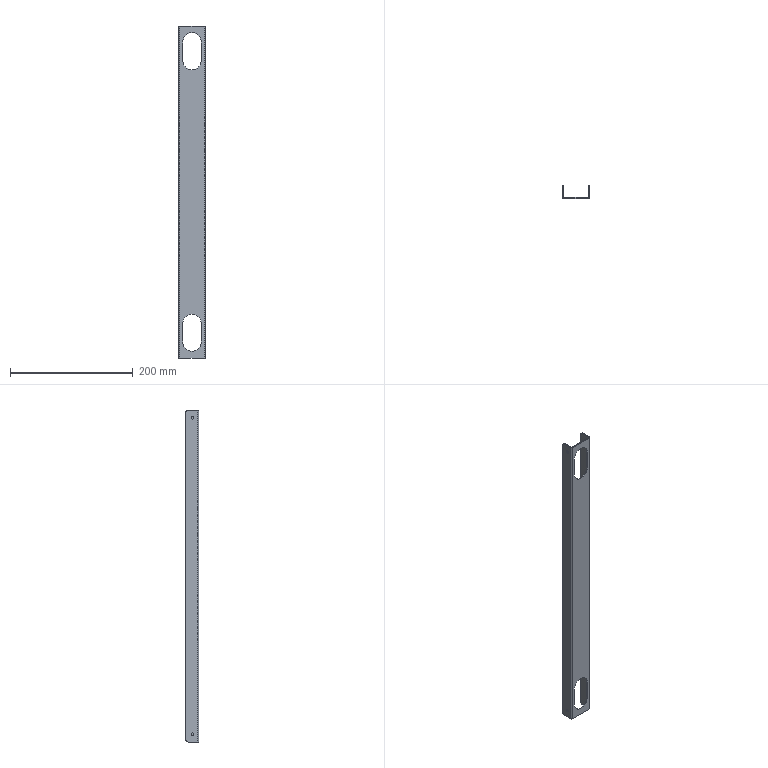Part | SolidWorks | features Cut 1, Fillet 1, FlatPattern 1, HoleWzd 1, SMBaseFlange 1, SheetMetal 1 | 1 solid | 40 faces | box 43 x 21.5 x 540 mm | volume 61599 mm3 | plane 22 | cylinder 18 | commonest cylinder face diameters 30 x6 4.5 x4 10 x4 0.6 x2 3.6 x2
STEP:
#1=CARTESIAN_POINT('',(20.,-1.5,71.));
#2=VERTEX_POINT('',#1);
#3=CARTESIAN_POINT('',(35.,-1.5,56.));
#4=VERTEX_POINT('',#3);
#5=CARTESIAN_POINT('',(20.,-1.5,56.));
#6=DIRECTION('',(0.,1.,0.));
#7=DIRECTION('',(0.,0.,1.));
#8=AXIS2_PLACEMENT_3D('',#5,#6,#7);
#9=CIRCLE('',#8,15.);
#10=EDGE_CURVE('',#2,#4,#9,.T.);
#11=ORIENTED_EDGE('',*,*,#10,.F.);
#12=CARTESIAN_POINT('',(20.,0.,71.));
#13=VERTEX_POINT('',#12);
#14=CARTESIAN_POINT('',(20.,-15.,71.));
#15=DIRECTION('',(0.,1.,0.));
#16=VECTOR('',#15,1000.);
#17=LINE('',#14,#16);
#18=EDGE_CURVE('',#2,#13,#17,.T.);
#19=ORIENTED_EDGE('',*,*,#18,.T.);
#20=CARTESIAN_POINT('',(35.,0.,56.));
#21=VERTEX_POINT('',#20);
#22=CARTESIAN_POINT('',(20.,0.,56.));
#23=DIRECTION('',(0.,1.,0.));
#24=DIRECTION('',(0.,0.,1.));
#25=AXIS2_PLACEMENT_3D('',#22,#23,#24);
#26=CIRCLE('',#25,15.);
#27=EDGE_CURVE('',#13,#21,#26,.T.);
#28=ORIENTED_EDGE('',*,*,#27,.T.);
#29=CARTESIAN_POINT('',(35.,-15.,56.));
#30=DIRECTION('',(0.,1.,0.));
#31=VECTOR('',#30,1000.);
#32=LINE('',#29,#31);
#33=EDGE_CURVE('',#4,#21,#32,.T.);
#34=ORIENTED_EDGE('',*,*,#33,.F.);
#35=EDGE_LOOP('',(#11,#19,#28,#34));
#36=FACE_OUTER_BOUND('',#35,.T.);
#37=CARTESIAN_POINT('',(20.,-15.,56.));
#38=DIRECTION('',(0.,1.,0.));
#39=DIRECTION('',(0.,0.,1.));
#40=AXIS2_PLACEMENT_3D('',#37,#38,#39);
#41=CYLINDRICAL_SURFACE('',#40,15.);
#42=ADVANCED_FACE('',(#36),#41,.F.);
#43=CARTESIAN_POINT('',(20.,-1.5,529.));
#44=VERTEX_POINT('',#43);
#45=CARTESIAN_POINT('',(35.,-1.5,514.));
#46=VERTEX_POINT('',#45);
#47=CARTESIAN_POINT('',(20.,-1.5,514.));
#48=DIRECTION('',(0.,1.,0.));
#49=DIRECTION('',(0.,0.,1.));
#50=AXIS2_PLACEMENT_3D('',#47,#48,#49);
#51=CIRCLE('',#50,15.);
#52=EDGE_CURVE('',#44,#46,#51,.T.);
#53=ORIENTED_EDGE('',*,*,#52,.F.);
#54=CARTESIAN_POINT('',(20.,0.,529.));
#55=VERTEX_POINT('',#54);
#56=CARTESIAN_POINT('',(20.,-15.,529.));
#57=DIRECTION('',(0.,1.,0.));
#58=VECTOR('',#57,1000.);
#59=LINE('',#56,#58);
#60=EDGE_CURVE('',#44,#55,#59,.T.);
#61=ORIENTED_EDGE('',*,*,#60,.T.);
#62=CARTESIAN_POINT('',(35.,0.,514.));
#63=VERTEX_POINT('',#62);
#64=CARTESIAN_POINT('',(20.,0.,514.));
#65=DIRECTION('',(0.,1.,0.));
#66=DIRECTION('',(0.,0.,-1.));
#67=AXIS2_PLACEMENT_3D('',#64,#65,#66);
#68=CIRCLE('',#67,15.);
#69=EDGE_CURVE('',#55,#63,#68,.T.);
#70=ORIENTED_EDGE('',*,*,#69,.T.);
#71=CARTESIAN_POINT('',(35.,-15.,514.));
#72=DIRECTION('',(0.,1.,0.));
#73=VECTOR('',#72,1000.);
#74=LINE('',#71,#73);
#75=EDGE_CURVE('',#46,#63,#74,.T.);
#76=ORIENTED_EDGE('',*,*,#75,.F.);
#77=EDGE_LOOP('',(#53,#61,#70,#76));
#78=FACE_OUTER_BOUND('',#77,.T.);
#79=CARTESIAN_POINT('',(20.,-15.,514.));
#80=DIRECTION('',(0.,1.,0.));
#81=DIRECTION('',(0.,0.,1.));
#82=AXIS2_PLACEMENT_3D('',#79,#80,#81);
#83=CYLINDRICAL_SURFACE('',#82,15.);
#84=ADVANCED_FACE('',(#78),#83,.F.);
#85=CARTESIAN_POINT('',(-1.5,8.5,529.75));
#86=VERTEX_POINT('',#85);
#87=CARTESIAN_POINT('',(-1.5,8.5,525.25));
#88=VERTEX_POINT('',#87);
#89=CARTESIAN_POINT('',(-1.5,8.5,527.5));
#90=DIRECTION('',(1.,0.,0.));
#91=DIRECTION('',(0.,0.,-1.));
#92=AXIS2_PLACEMENT_3D('',#89,#90,#91);
#93=CIRCLE('',#92,2.25);
#94=EDGE_CURVE('',#86,#88,#93,.T.);
#95=ORIENTED_EDGE('',*,*,#94,.F.);
#96=CARTESIAN_POINT('',(0.,8.5,529.75));
#97=VERTEX_POINT('',#96);
#98=CARTESIAN_POINT('',(0.,8.5,529.75));
#99=DIRECTION('',(1.,0.,0.));
#100=VECTOR('',#99,1000.);
#101=LINE('',#98,#100);
#102=EDGE_CURVE('',#86,#97,#101,.T.);
#103=ORIENTED_EDGE('',*,*,#102,.T.);
#104=CARTESIAN_POINT('',(0.,8.5,525.25));
#105=VERTEX_POINT('',#104);
#106=CARTESIAN_POINT('',(0.,8.5,527.5));
#107=DIRECTION('',(1.,0.,0.));
#108=DIRECTION('',(0.,0.,-1.));
#109=AXIS2_PLACEMENT_3D('',#106,#107,#108);
#110=CIRCLE('',#109,2.25);
#111=EDGE_CURVE('',#97,#105,#110,.T.);
#112=ORIENTED_EDGE('',*,*,#111,.T.);
#113=CARTESIAN_POINT('',(0.,8.5,525.25));
#114=DIRECTION('',(1.,0.,0.));
#115=VECTOR('',#114,1000.);
#116=LINE('',#113,#115);
#117=EDGE_CURVE('',#88,#105,#116,.T.);
#118=ORIENTED_EDGE('',*,*,#117,.F.);
#119=EDGE_LOOP('',(#95,#103,#112,#118));
#120=FACE_OUTER_BOUND('',#119,.T.);
#121=CARTESIAN_POINT('',(0.,8.5,527.5));
#122=DIRECTION('',(1.,0.,0.));
#123=DIRECTION('',(0.,0.,-1.));
#124=AXIS2_PLACEMENT_3D('',#121,#122,#123);
#125=CYLINDRICAL_SURFACE('',#124,2.25);
#126=ADVANCED_FACE('',(#120),#125,.F.);
#127=CARTESIAN_POINT('',(-1.5,8.5,14.75));
#128=VERTEX_POINT('',#127);
#129=CARTESIAN_POINT('',(-1.5,8.5,10.25));
#130=VERTEX_POINT('',#129);
#131=CARTESIAN_POINT('',(-1.5,8.5,12.5));
#132=DIRECTION('',(1.,0.,0.));
#133=DIRECTION('',(0.,0.,-1.));
#134=AXIS2_PLACEMENT_3D('',#131,#132,#133);
#135=CIRCLE('',#134,2.25);
#136=EDGE_CURVE('',#128,#130,#135,.T.);
#137=ORIENTED_EDGE('',*,*,#136,.F.);
#138=CARTESIAN_POINT('',(0.,8.5,14.75));
#139=VERTEX_POINT('',#138);
#140=CARTESIAN_POINT('',(0.,8.5,14.75));
#141=DIRECTION('',(1.,0.,0.));
#142=VECTOR('',#141,1000.);
#143=LINE('',#140,#142);
#144=EDGE_CURVE('',#128,#139,#143,.T.);
#145=ORIENTED_EDGE('',*,*,#144,.T.);
#146=CARTESIAN_POINT('',(0.,8.5,10.25));
#147=VERTEX_POINT('',#146);
#148=CARTESIAN_POINT('',(0.,8.5,12.5));
#149=DIRECTION('',(1.,0.,0.));
#150=DIRECTION('',(0.,0.,-1.));
#151=AXIS2_PLACEMENT_3D('',#148,#149,#150);
#152=CIRCLE('',#151,2.25);
#153=EDGE_CURVE('',#139,#147,#152,.T.);
#154=ORIENTED_EDGE('',*,*,#153,.T.);
#155=CARTESIAN_POINT('',(0.,8.5,10.25));
#156=DIRECTION('',(1.,0.,0.));
#157=VECTOR('',#156,1000.);
#158=LINE('',#155,#157);
#159=EDGE_CURVE('',#130,#147,#158,.T.);
#160=ORIENTED_EDGE('',*,*,#159,.F.);
#161=EDGE_LOOP('',(#137,#145,#154,#160));
#162=FACE_OUTER_BOUND('',#161,.T.);
#163=CARTESIAN_POINT('',(0.,8.5,12.5));
#164=DIRECTION('',(1.,0.,0.));
#165=DIRECTION('',(0.,0.,-1.));
#166=AXIS2_PLACEMENT_3D('',#163,#164,#165);
#167=CYLINDRICAL_SURFACE('',#166,2.25);
#168=ADVANCED_FACE('',(#162),#167,.F.);
#169=CARTESIAN_POINT('',(0.3,0.,540.));
#170=VERTEX_POINT('',#169);
#171=CARTESIAN_POINT('',(0.3,-1.5,540.));
#172=VERTEX_POINT('',#171);
#173=CARTESIAN_POINT('',(0.3,0.,540.));
#174=DIRECTION('',(0.,-1.,0.));
#175=VECTOR('',#174,1000.);
#176=LINE('',#173,#175);
#177=EDGE_CURVE('',#170,#172,#176,.T.);
#178=ORIENTED_EDGE('',*,*,#177,.F.);
#179=CARTESIAN_POINT('',(0.,0.3,540.));
#180=VERTEX_POINT('',#179);
#181=CARTESIAN_POINT('',(0.3,0.3,540.));
#182=DIRECTION('',(0.,0.,1.));
#183=DIRECTION('',(-1.,0.,0.));
#184=AXIS2_PLACEMENT_3D('',#181,#182,#183);
#185=CIRCLE('',#184,0.3);
#186=EDGE_CURVE('',#180,#170,#185,.T.);
#187=ORIENTED_EDGE('',*,*,#186,.F.);
#188=CARTESIAN_POINT('',(-1.5,0.3,540.));
#189=VERTEX_POINT('',#188);
#190=CARTESIAN_POINT('',(-1.5,0.3,540.));
#191=DIRECTION('',(1.,0.,0.));
#192=VECTOR('',#191,1000.);
#193=LINE('',#190,#192);
#194=EDGE_CURVE('',#189,#180,#193,.T.);
#195=ORIENTED_EDGE('',*,*,#194,.F.);
#196=CARTESIAN_POINT('',(0.3,0.3,540.));
#197=DIRECTION('',(0.,0.,1.));
#198=DIRECTION('',(1.,0.,0.));
#199=AXIS2_PLACEMENT_3D('',#196,#197,#198);
#200=CIRCLE('',#199,1.8);
#201=EDGE_CURVE('',#189,#172,#200,.T.);
#202=ORIENTED_EDGE('',*,*,#201,.T.);
#203=EDGE_LOOP('',(#178,#187,#195,#202));
#204=FACE_OUTER_BOUND('',#203,.T.);
#205=CARTESIAN_POINT('',(0.3,0.,540.));
#206=DIRECTION('',(0.,0.,1.));
#207=DIRECTION('',(1.,0.,0.));
#208=AXIS2_PLACEMENT_3D('',#205,#206,#207);
#209=PLANE('',#208);
#210=ADVANCED_FACE('',(#204),#209,.T.);
#211=CARTESIAN_POINT('',(39.7,0.,540.));
#212=VERTEX_POINT('',#211);
#213=CARTESIAN_POINT('',(0.,0.,540.));
#214=DIRECTION('',(1.,0.,0.));
#215=VECTOR('',#214,1000.);
#216=LINE('',#213,#215);
#217=EDGE_CURVE('',#170,#212,#216,.T.);
#218=ORIENTED_EDGE('',*,*,#217,.F.);
#219=ORIENTED_EDGE('',*,*,#177,.T.);
#220=CARTESIAN_POINT('',(39.7,-1.5,540.));
#221=VERTEX_POINT('',#220);
#222=CARTESIAN_POINT('',(0.,-1.5,540.));
#223=DIRECTION('',(1.,0.,0.));
#224=VECTOR('',#223,1000.);
#225=LINE('',#222,#224);
#226=EDGE_CURVE('',#172,#221,#225,.T.);
#227=ORIENTED_EDGE('',*,*,#226,.T.);
#228=CARTESIAN_POINT('',(39.7,-1.5,540.));
#229=DIRECTION('',(0.,1.,0.));
#230=VECTOR('',#229,1000.);
#231=LINE('',#228,#230);
#232=EDGE_CURVE('',#221,#212,#231,.T.);
#233=ORIENTED_EDGE('',*,*,#232,.T.);
#234=EDGE_LOOP('',(#218,#219,#227,#233));
#235=FACE_OUTER_BOUND('',#234,.T.);
#236=CARTESIAN_POINT('',(-1.5,0.3,540.));
#237=DIRECTION('',(0.,0.,1.));
#238=DIRECTION('',(1.,0.,0.));
#239=AXIS2_PLACEMENT_3D('',#236,#237,#238);
#240=PLANE('',#239);
#241=ADVANCED_FACE('',(#235),#240,.T.);
#242=CARTESIAN_POINT('',(0.,0.3,0.));
#243=VERTEX_POINT('',#242);
#244=CARTESIAN_POINT('',(-1.5,0.3,0.));
#245=VERTEX_POINT('',#244);
#246=CARTESIAN_POINT('',(0.,0.3,0.));
#247=DIRECTION('',(-1.,0.,0.));
#248=VECTOR('',#247,1000.);
#249=LINE('',#246,#248);
#250=EDGE_CURVE('',#243,#245,#249,.T.);
#251=ORIENTED_EDGE('',*,*,#250,.F.);
#252=CARTESIAN_POINT('',(0.3,0.,0.));
#253=VERTEX_POINT('',#252);
#254=CARTESIAN_POINT('',(0.3,0.3,0.));
#255=DIRECTION('',(0.,0.,1.));
#256=DIRECTION('',(-1.,0.,0.));
#257=AXIS2_PLACEMENT_3D('',#254,#255,#256);
#258=CIRCLE('',#257,0.3);
#259=EDGE_CURVE('',#243,#253,#258,.T.);
#260=ORIENTED_EDGE('',*,*,#259,.T.);
#261=CARTESIAN_POINT('',(0.3,-1.5,0.));
#262=VERTEX_POINT('',#261);
#263=CARTESIAN_POINT('',(0.3,-1.5,0.));
#264=DIRECTION('',(0.,1.,0.));
#265=VECTOR('',#264,1000.);
#266=LINE('',#263,#265);
#267=EDGE_CURVE('',#262,#253,#266,.T.);
#268=ORIENTED_EDGE('',*,*,#267,.F.);
#269=CARTESIAN_POINT('',(0.3,0.3,0.));
#270=DIRECTION('',(0.,0.,1.));
#271=DIRECTION('',(1.,0.,0.));
#272=AXIS2_PLACEMENT_3D('',#269,#270,#271);
#273=CIRCLE('',#272,1.8);
#274=EDGE_CURVE('',#245,#262,#273,.T.);
#275=ORIENTED_EDGE('',*,*,#274,.F.);
#276=EDGE_LOOP('',(#251,#260,#268,#275));
#277=FACE_OUTER_BOUND('',#276,.T.);
#278=CARTESIAN_POINT('',(0.,0.3,0.));
#279=DIRECTION('',(0.,0.,-1.));
#280=DIRECTION('',(-1.,0.,0.));
#281=AXIS2_PLACEMENT_3D('',#278,#279,#280);
#282=PLANE('',#281);
#283=ADVANCED_FACE('',(#277),#282,.T.);
#284=CARTESIAN_POINT('',(-1.5,15.,0.));
#285=VERTEX_POINT('',#284);
#286=CARTESIAN_POINT('',(-1.5,0.,0.));
#287=DIRECTION('',(0.,-1.,0.));
#288=VECTOR('',#287,1000.);
#289=LINE('',#286,#288);
#290=EDGE_CURVE('',#285,#245,#289,.T.);
#291=ORIENTED_EDGE('',*,*,#290,.F.);
#292=CARTESIAN_POINT('',(0.,15.,0.));
#293=VERTEX_POINT('',#292);
#294=CARTESIAN_POINT('',(0.3,15.,0.));
#295=DIRECTION('',(1.,0.,0.));
#296=VECTOR('',#295,1000.);
#297=LINE('',#294,#296);
#298=EDGE_CURVE('',#285,#293,#297,.T.);
#299=ORIENTED_EDGE('',*,*,#298,.T.);
#300=CARTESIAN_POINT('',(0.,0.,0.));
#301=DIRECTION('',(0.,-1.,0.));
#302=VECTOR('',#301,1000.);
#303=LINE('',#300,#302);
#304=EDGE_CURVE('',#293,#243,#303,.T.);
#305=ORIENTED_EDGE('',*,*,#304,.T.);
#306=ORIENTED_EDGE('',*,*,#250,.T.);
#307=EDGE_LOOP('',(#291,#299,#305,#306));
#308=FACE_OUTER_BOUND('',#307,.T.);
#309=CARTESIAN_POINT('',(0.3,-1.5,0.));
#310=DIRECTION('',(0.,0.,-1.));
#311=DIRECTION('',(-1.,0.,0.));
#312=AXIS2_PLACEMENT_3D('',#309,#310,#311);
#313=PLANE('',#312);
#314=ADVANCED_FACE('',(#308),#313,.T.);
#315=CARTESIAN_POINT('',(40.,0.3,540.));
#316=VERTEX_POINT('',#315);
#317=CARTESIAN_POINT('',(41.5,0.3,540.));
#318=VERTEX_POINT('',#317);
#319=CARTESIAN_POINT('',(40.,0.3,540.));
#320=DIRECTION('',(1.,0.,0.));
#321=VECTOR('',#320,1000.);
#322=LINE('',#319,#321);
#323=EDGE_CURVE('',#316,#318,#322,.T.);
#324=ORIENTED_EDGE('',*,*,#323,.F.);
#325=CARTESIAN_POINT('',(39.7,0.3,540.));
#326=DIRECTION('',(0.,0.,1.));
#327=DIRECTION('',(-1.,0.,0.));
#328=AXIS2_PLACEMENT_3D('',#325,#326,#327);
#329=CIRCLE('',#328,0.3);
#330=EDGE_CURVE('',#212,#316,#329,.T.);
#331=ORIENTED_EDGE('',*,*,#330,.F.);
#332=ORIENTED_EDGE('',*,*,#232,.F.);
#333=CARTESIAN_POINT('',(39.7,0.3,540.));
#334=DIRECTION('',(0.,0.,1.));
#335=DIRECTION('',(1.,0.,0.));
#336=AXIS2_PLACEMENT_3D('',#333,#334,#335);
#337=CIRCLE('',#336,1.8);
#338=EDGE_CURVE('',#221,#318,#337,.T.);
#339=ORIENTED_EDGE('',*,*,#338,.T.);
#340=EDGE_LOOP('',(#324,#331,#332,#339));
#341=FACE_OUTER_BOUND('',#340,.T.);
#342=CARTESIAN_POINT('',(40.,0.3,540.));
#343=DIRECTION('',(0.,0.,1.));
#344=DIRECTION('',(1.,0.,0.));
#345=AXIS2_PLACEMENT_3D('',#342,#343,#344);
#346=PLANE('',#345);
#347=ADVANCED_FACE('',(#341),#346,.T.);
#348=CARTESIAN_POINT('',(41.5,15.,540.));
#349=VERTEX_POINT('',#348);
#350=CARTESIAN_POINT('',(41.5,0.,540.));
#351=DIRECTION('',(0.,1.,0.));
#352=VECTOR('',#351,1000.);
#353=LINE('',#350,#352);
#354=EDGE_CURVE('',#318,#349,#353,.T.);
#355=ORIENTED_EDGE('',*,*,#354,.T.);
#356=CARTESIAN_POINT('',(40.,15.,540.));
#357=VERTEX_POINT('',#356);
#358=CARTESIAN_POINT('',(39.7,15.,540.));
#359=DIRECTION('',(-1.,0.,0.));
#360=VECTOR('',#359,1000.);
#361=LINE('',#358,#360);
#362=EDGE_CURVE('',#349,#357,#361,.T.);
#363=ORIENTED_EDGE('',*,*,#362,.T.);
#364=CARTESIAN_POINT('',(40.,0.,540.));
#365=DIRECTION('',(0.,1.,0.));
#366=VECTOR('',#365,1000.);
#367=LINE('',#364,#366);
#368=EDGE_CURVE('',#316,#357,#367,.T.);
#369=ORIENTED_EDGE('',*,*,#368,.F.);
#370=ORIENTED_EDGE('',*,*,#323,.T.);
#371=EDGE_LOOP('',(#355,#363,#369,#370));
#372=FACE_OUTER_BOUND('',#371,.T.);
#373=CARTESIAN_POINT('',(39.7,-1.5,540.));
#374=DIRECTION('',(0.,0.,1.));
#375=DIRECTION('',(1.,0.,0.));
#376=AXIS2_PLACEMENT_3D('',#373,#374,#375);
#377=PLANE('',#376);
#378=ADVANCED_FACE('',(#372),#377,.T.);
#379=CARTESIAN_POINT('',(39.7,0.,0.));
#380=VERTEX_POINT('',#379);
#381=CARTESIAN_POINT('',(39.7,-1.5,0.));
#382=VERTEX_POINT('',#381);
#383=CARTESIAN_POINT('',(39.7,0.,0.));
#384=DIRECTION('',(0.,-1.,0.));
#385=VECTOR('',#384,1000.);
#386=LINE('',#383,#385);
#387=EDGE_CURVE('',#380,#382,#386,.T.);
#388=ORIENTED_EDGE('',*,*,#387,.F.);
#389=CARTESIAN_POINT('',(40.,0.3,0.));
#390=VERTEX_POINT('',#389);
#391=CARTESIAN_POINT('',(39.7,0.3,0.));
#392=DIRECTION('',(0.,0.,1.));
#393=DIRECTION('',(-1.,0.,0.));
#394=AXIS2_PLACEMENT_3D('',#391,#392,#393);
#395=CIRCLE('',#394,0.3);
#396=EDGE_CURVE('',#380,#390,#395,.T.);
#397=ORIENTED_EDGE('',*,*,#396,.T.);
#398=CARTESIAN_POINT('',(41.5,0.3,0.));
#399=VERTEX_POINT('',#398);
#400=CARTESIAN_POINT('',(41.5,0.3,0.));
#401=DIRECTION('',(-1.,0.,0.));
#402=VECTOR('',#401,1000.);
#403=LINE('',#400,#402);
#404=EDGE_CURVE('',#399,#390,#403,.T.);
#405=ORIENTED_EDGE('',*,*,#404,.F.);
#406=CARTESIAN_POINT('',(39.7,0.3,0.));
#407=DIRECTION('',(0.,0.,1.));
#408=DIRECTION('',(1.,0.,0.));
#409=AXIS2_PLACEMENT_3D('',#406,#407,#408);
#410=CIRCLE('',#409,1.8);
#411=EDGE_CURVE('',#382,#399,#410,.T.);
#412=ORIENTED_EDGE('',*,*,#411,.F.);
#413=EDGE_LOOP('',(#388,#397,#405,#412));
#414=FACE_OUTER_BOUND('',#413,.T.);
#415=CARTESIAN_POINT('',(39.7,0.,0.));
#416=DIRECTION('',(0.,0.,-1.));
#417=DIRECTION('',(-1.,0.,0.));
#418=AXIS2_PLACEMENT_3D('',#415,#416,#417);
#419=PLANE('',#418);
#420=ADVANCED_FACE('',(#414),#419,.T.);
#421=CARTESIAN_POINT('',(0.,0.,0.));
#422=DIRECTION('',(1.,0.,0.));
#423=VECTOR('',#422,1000.);
#424=LINE('',#421,#423);
#425=EDGE_CURVE('',#253,#380,#424,.T.);
#426=ORIENTED_EDGE('',*,*,#425,.T.);
#427=ORIENTED_EDGE('',*,*,#387,.T.);
#428=CARTESIAN_POINT('',(0.,-1.5,0.));
#429=DIRECTION('',(1.,0.,0.));
#430=VECTOR('',#429,1000.);
#431=LINE('',#428,#430);
#432=EDGE_CURVE('',#262,#382,#431,.T.);
#433=ORIENTED_EDGE('',*,*,#432,.F.);
#434=ORIENTED_EDGE('',*,*,#267,.T.);
#435=EDGE_LOOP('',(#426,#427,#433,#434));
#436=FACE_OUTER_BOUND('',#435,.T.);
#437=CARTESIAN_POINT('',(41.5,0.3,0.));
#438=DIRECTION('',(0.,0.,-1.));
#439=DIRECTION('',(-1.,0.,0.));
#440=AXIS2_PLACEMENT_3D('',#437,#438,#439);
#441=PLANE('',#440);
#442=ADVANCED_FACE('',(#436),#441,.T.);
#443=CARTESIAN_POINT('',(41.5,20.,535.));
#444=VERTEX_POINT('',#443);
#445=CARTESIAN_POINT('',(41.5,20.,5.));
#446=VERTEX_POINT('',#445);
#447=CARTESIAN_POINT('',(41.5,20.,540.));
#448=DIRECTION('',(0.,0.,-1.));
#449=VECTOR('',#448,1000.);
#450=LINE('',#447,#449);
#451=EDGE_CURVE('',#444,#446,#450,.T.);
#452=ORIENTED_EDGE('',*,*,#451,.F.);
#453=CARTESIAN_POINT('',(41.5,15.,535.));
#454=DIRECTION('',(1.,0.,0.));
#455=DIRECTION('',(0.,0.,1.));
#456=AXIS2_PLACEMENT_3D('',#453,#454,#455);
#457=CIRCLE('',#456,5.);
#458=EDGE_CURVE('',#444,#349,#457,.T.);
#459=ORIENTED_EDGE('',*,*,#458,.T.);
#460=ORIENTED_EDGE('',*,*,#354,.F.);
#461=CARTESIAN_POINT('',(41.5,0.3,540.));
#462=DIRECTION('',(0.,0.,-1.));
#463=VECTOR('',#462,1000.);
#464=LINE('',#461,#463);
#465=EDGE_CURVE('',#318,#399,#464,.T.);
#466=ORIENTED_EDGE('',*,*,#465,.T.);
#467=CARTESIAN_POINT('',(41.5,15.,0.));
#468=VERTEX_POINT('',#467);
#469=CARTESIAN_POINT('',(41.5,0.,0.));
#470=DIRECTION('',(0.,1.,0.));
#471=VECTOR('',#470,1000.);
#472=LINE('',#469,#471);
#473=EDGE_CURVE('',#399,#468,#472,.T.);
#474=ORIENTED_EDGE('',*,*,#473,.T.);
#475=CARTESIAN_POINT('',(41.5,15.,5.));
#476=DIRECTION('',(1.,0.,0.));
#477=DIRECTION('',(0.,0.,1.));
#478=AXIS2_PLACEMENT_3D('',#475,#476,#477);
#479=CIRCLE('',#478,5.);
#480=EDGE_CURVE('',#468,#446,#479,.T.);
#481=ORIENTED_EDGE('',*,*,#480,.T.);
#482=EDGE_LOOP('',(#452,#459,#460,#466,#474,#481));
#483=FACE_OUTER_BOUND('',#482,.T.);
#484=CARTESIAN_POINT('',(41.5,0.,540.));
#485=DIRECTION('',(-1.,0.,0.));
#486=DIRECTION('',(0.,0.,1.));
#487=AXIS2_PLACEMENT_3D('',#484,#485,#486);
#488=PLANE('',#487);
#489=ADVANCED_FACE('',(#483),#488,.F.);
#490=CARTESIAN_POINT('',(40.,20.,535.));
#491=VERTEX_POINT('',#490);
#492=CARTESIAN_POINT('',(40.,20.,5.));
#493=VERTEX_POINT('',#492);
#494=CARTESIAN_POINT('',(40.,20.,540.));
#495=DIRECTION('',(0.,0.,-1.));
#496=VECTOR('',#495,1000.);
#497=LINE('',#494,#496);
#498=EDGE_CURVE('',#491,#493,#497,.T.);
#499=ORIENTED_EDGE('',*,*,#498,.F.);
#500=CARTESIAN_POINT('',(40.,20.,535.));
#501=DIRECTION('',(1.,0.,0.));
#502=VECTOR('',#501,1000.);
#503=LINE('',#500,#502);
#504=EDGE_CURVE('',#491,#444,#503,.T.);
#505=ORIENTED_EDGE('',*,*,#504,.T.);
#506=ORIENTED_EDGE('',*,*,#451,.T.);
#507=CARTESIAN_POINT('',(40.,20.,5.));
#508=DIRECTION('',(-1.,0.,0.));
#509=VECTOR('',#508,1000.);
#510=LINE('',#507,#509);
#511=EDGE_CURVE('',#446,#493,#510,.T.);
#512=ORIENTED_EDGE('',*,*,#511,.T.);
#513=EDGE_LOOP('',(#499,#505,#506,#512));
#514=FACE_OUTER_BOUND('',#513,.T.);
#515=CARTESIAN_POINT('',(40.,20.,540.));
#516=DIRECTION('',(0.,1.,0.));
#517=DIRECTION('',(0.,0.,1.));
#518=AXIS2_PLACEMENT_3D('',#515,#516,#517);
#519=PLANE('',#518);
#520=ADVANCED_FACE('',(#514),#519,.T.);
#521=ORIENTED_EDGE('',*,*,#368,.T.);
#522=CARTESIAN_POINT('',(40.,15.,535.));
#523=DIRECTION('',(-1.,0.,0.));
#524=DIRECTION('',(0.,0.,1.));
#525=AXIS2_PLACEMENT_3D('',#522,#523,#524);
#526=CIRCLE('',#525,5.);
#527=EDGE_CURVE('',#357,#491,#526,.T.);
#528=ORIENTED_EDGE('',*,*,#527,.T.);
#529=ORIENTED_EDGE('',*,*,#498,.T.);
#530=CARTESIAN_POINT('',(40.,15.,0.));
#531=VERTEX_POINT('',#530);
#532=CARTESIAN_POINT('',(40.,15.,5.));
#533=DIRECTION('',(-1.,0.,0.));
#534=DIRECTION('',(0.,0.,1.));
#535=AXIS2_PLACEMENT_3D('',#532,#533,#534);
#536=CIRCLE('',#535,5.);
#537=EDGE_CURVE('',#493,#531,#536,.T.);
#538=ORIENTED_EDGE('',*,*,#537,.T.);
#539=CARTESIAN_POINT('',(40.,0.,0.));
#540=DIRECTION('',(0.,1.,0.));
#541=VECTOR('',#540,1000.);
#542=LINE('',#539,#541);
#543=EDGE_CURVE('',#390,#531,#542,.T.);
#544=ORIENTED_EDGE('',*,*,#543,.F.);
#545=CARTESIAN_POINT('',(40.,0.3,540.));
#546=DIRECTION('',(0.,0.,-1.));
#547=VECTOR('',#546,1000.);
#548=LINE('',#545,#547);
#549=EDGE_CURVE('',#316,#390,#548,.T.);
#550=ORIENTED_EDGE('',*,*,#549,.F.);
#551=EDGE_LOOP('',(#521,#528,#529,#538,#544,#550));
#552=FACE_OUTER_BOUND('',#551,.T.);
#553=CARTESIAN_POINT('',(40.,0.,540.));
#554=DIRECTION('',(-1.,0.,0.));
#555=DIRECTION('',(0.,0.,1.));
#556=AXIS2_PLACEMENT_3D('',#553,#554,#555);
#557=PLANE('',#556);
#558=ADVANCED_FACE('',(#552),#557,.T.);
#559=ORIENTED_EDGE('',*,*,#396,.F.);
#560=CARTESIAN_POINT('',(39.7,0.,540.));
#561=DIRECTION('',(0.,0.,-1.));
#562=VECTOR('',#561,1000.);
#563=LINE('',#560,#562);
#564=EDGE_CURVE('',#212,#380,#563,.T.);
#565=ORIENTED_EDGE('',*,*,#564,.F.);
#566=ORIENTED_EDGE('',*,*,#330,.T.);
#567=ORIENTED_EDGE('',*,*,#549,.T.);
#568=EDGE_LOOP('',(#559,#565,#566,#567));
#569=FACE_OUTER_BOUND('',#568,.T.);
#570=CARTESIAN_POINT('',(39.7,0.3,540.));
#571=DIRECTION('',(0.,0.,-1.));
#572=DIRECTION('',(-1.,0.,0.));
#573=AXIS2_PLACEMENT_3D('',#570,#571,#572);
#574=CYLINDRICAL_SURFACE('',#573,0.3);
#575=ADVANCED_FACE('',(#569),#574,.F.);
#576=CARTESIAN_POINT('',(35.,0.,26.));
#577=VERTEX_POINT('',#576);
#578=CARTESIAN_POINT('',(5.,0.,26.));
#579=VERTEX_POINT('',#578);
#580=CARTESIAN_POINT('',(20.,0.,26.));
#581=DIRECTION('',(0.,1.,0.));
#582=DIRECTION('',(0.,0.,1.));
#583=AXIS2_PLACEMENT_3D('',#580,#581,#582);
#584=CIRCLE('',#583,15.);
#585=EDGE_CURVE('',#577,#579,#584,.T.);
#586=ORIENTED_EDGE('',*,*,#585,.F.);
#587=CARTESIAN_POINT('',(35.,0.,26.));
#588=DIRECTION('',(0.,0.,-1.));
#589=VECTOR('',#588,1000.);
#590=LINE('',#587,#589);
#591=EDGE_CURVE('',#21,#577,#590,.T.);
#592=ORIENTED_EDGE('',*,*,#591,.F.);
#593=ORIENTED_EDGE('',*,*,#27,.F.);
#594=CARTESIAN_POINT('',(5.,0.,56.));
#595=VERTEX_POINT('',#594);
#596=CARTESIAN_POINT('',(20.,0.,56.));
#597=DIRECTION('',(0.,1.,0.));
#598=DIRECTION('',(0.,0.,1.));
#599=AXIS2_PLACEMENT_3D('',#596,#597,#598);
#600=CIRCLE('',#599,15.);
#601=EDGE_CURVE('',#595,#13,#600,.T.);
#602=ORIENTED_EDGE('',*,*,#601,.F.);
#603=CARTESIAN_POINT('',(5.,0.,26.));
#604=DIRECTION('',(0.,0.,1.));
#605=VECTOR('',#604,1000.);
#606=LINE('',#603,#605);
#607=EDGE_CURVE('',#579,#595,#606,.T.);
#608=ORIENTED_EDGE('',*,*,#607,.F.);
#609=EDGE_LOOP('',(#586,#592,#593,#602,#608));
#610=FACE_BOUND('',#609,.T.);
#611=CARTESIAN_POINT('',(5.,0.,514.));
#612=VERTEX_POINT('',#611);
#613=CARTESIAN_POINT('',(20.,0.,514.));
#614=DIRECTION('',(0.,1.,0.));
#615=DIRECTION('',(0.,0.,-1.));
#616=AXIS2_PLACEMENT_3D('',#613,#614,#615);
#617=CIRCLE('',#616,15.);
#618=EDGE_CURVE('',#612,#55,#617,.T.);
#619=ORIENTED_EDGE('',*,*,#618,.F.);
#620=CARTESIAN_POINT('',(5.,0.,484.));
#621=VERTEX_POINT('',#620);
#622=CARTESIAN_POINT('',(5.,0.,514.));
#623=DIRECTION('',(0.,0.,1.));
#624=VECTOR('',#623,1000.);
#625=LINE('',#622,#624);
#626=EDGE_CURVE('',#621,#612,#625,.T.);
#627=ORIENTED_EDGE('',*,*,#626,.F.);
#628=CARTESIAN_POINT('',(35.,0.,484.));
#629=VERTEX_POINT('',#628);
#630=CARTESIAN_POINT('',(20.,0.,484.));
#631=DIRECTION('',(0.,1.,0.));
#632=DIRECTION('',(0.,0.,-1.));
#633=AXIS2_PLACEMENT_3D('',#630,#631,#632);
#634=CIRCLE('',#633,15.);
#635=EDGE_CURVE('',#629,#621,#634,.T.);
#636=ORIENTED_EDGE('',*,*,#635,.F.);
#637=CARTESIAN_POINT('',(35.,0.,514.));
#638=DIRECTION('',(0.,0.,-1.));
#639=VECTOR('',#638,1000.);
#640=LINE('',#637,#639);
#641=EDGE_CURVE('',#63,#629,#640,.T.);
#642=ORIENTED_EDGE('',*,*,#641,.F.);
#643=ORIENTED_EDGE('',*,*,#69,.F.);
#644=EDGE_LOOP('',(#619,#627,#636,#642,#643));
#645=FACE_BOUND('',#644,.T.);
#646=ORIENTED_EDGE('',*,*,#425,.F.);
#647=CARTESIAN_POINT('',(0.3,0.,540.));
#648=DIRECTION('',(0.,0.,-1.));
#649=VECTOR('',#648,1000.);
#650=LINE('',#647,#649);
#651=EDGE_CURVE('',#170,#253,#650,.T.);
#652=ORIENTED_EDGE('',*,*,#651,.F.);
#653=ORIENTED_EDGE('',*,*,#217,.T.);
#654=ORIENTED_EDGE('',*,*,#564,.T.);
#655=EDGE_LOOP('',(#646,#652,#653,#654));
#656=FACE_OUTER_BOUND('',#655,.T.);
#657=CARTESIAN_POINT('',(0.,0.,540.));
#658=DIRECTION('',(0.,1.,0.));
#659=DIRECTION('',(0.,0.,1.));
#660=AXIS2_PLACEMENT_3D('',#657,#658,#659);
#661=PLANE('',#660);
#662=ADVANCED_FACE('',(#610,#645,#656),#661,.T.);
#663=ORIENTED_EDGE('',*,*,#259,.F.);
#664=CARTESIAN_POINT('',(0.,0.3,540.));
#665=DIRECTION('',(0.,0.,-1.));
#666=VECTOR('',#665,1000.);
#667=LINE('',#664,#666);
#668=EDGE_CURVE('',#180,#243,#667,.T.);
#669=ORIENTED_EDGE('',*,*,#668,.F.);
#670=ORIENTED_EDGE('',*,*,#186,.T.);
#671=ORIENTED_EDGE('',*,*,#651,.T.);
#672=EDGE_LOOP('',(#663,#669,#670,#671));
#673=FACE_OUTER_BOUND('',#672,.T.);
#674=CARTESIAN_POINT('',(0.3,0.3,540.));
#675=DIRECTION('',(0.,0.,-1.));
#676=DIRECTION('',(-1.,0.,0.));
#677=AXIS2_PLACEMENT_3D('',#674,#675,#676);
#678=CYLINDRICAL_SURFACE('',#677,0.3);
#679=ADVANCED_FACE('',(#673),#678,.F.);
#680=CARTESIAN_POINT('',(0.,8.5,527.5));
#681=DIRECTION('',(1.,0.,0.));
#682=DIRECTION('',(0.,0.,-1.));
#683=AXIS2_PLACEMENT_3D('',#680,#681,#682);
#684=CIRCLE('',#683,2.25);
#685=EDGE_CURVE('',#105,#97,#684,.T.);
#686=ORIENTED_EDGE('',*,*,#685,.F.);
#687=ORIENTED_EDGE('',*,*,#111,.F.);
#688=EDGE_LOOP('',(#686,#687));
#689=FACE_BOUND('',#688,.T.);
#690=CARTESIAN_POINT('',(0.,8.5,12.5));
#691=DIRECTION('',(1.,0.,0.));
#692=DIRECTION('',(0.,0.,-1.));
#693=AXIS2_PLACEMENT_3D('',#690,#691,#692);
#694=CIRCLE('',#693,2.25);
#695=EDGE_CURVE('',#147,#139,#694,.T.);
#696=ORIENTED_EDGE('',*,*,#695,.F.);
#697=ORIENTED_EDGE('',*,*,#153,.F.);
#698=EDGE_LOOP('',(#696,#697));
#699=FACE_BOUND('',#698,.T.);
#700=CARTESIAN_POINT('',(0.,20.,535.));
#701=VERTEX_POINT('',#700);
#702=CARTESIAN_POINT('',(0.,20.,5.));
#703=VERTEX_POINT('',#702);
#704=CARTESIAN_POINT('',(0.,20.,540.));
#705=DIRECTION('',(0.,0.,-1.));
#706=VECTOR('',#705,1000.);
#707=LINE('',#704,#706);
#708=EDGE_CURVE('',#701,#703,#707,.T.);
#709=ORIENTED_EDGE('',*,*,#708,.F.);
#710=CARTESIAN_POINT('',(0.,15.,540.));
#711=VERTEX_POINT('',#710);
#712=CARTESIAN_POINT('',(0.,15.,535.));
#713=DIRECTION('',(1.,0.,0.));
#714=DIRECTION('',(0.,0.,-1.));
#715=AXIS2_PLACEMENT_3D('',#712,#713,#714);
#716=CIRCLE('',#715,5.);
#717=EDGE_CURVE('',#701,#711,#716,.T.);
#718=ORIENTED_EDGE('',*,*,#717,.T.);
#719=CARTESIAN_POINT('',(0.,0.,540.));
#720=DIRECTION('',(0.,-1.,0.));
#721=VECTOR('',#720,1000.);
#722=LINE('',#719,#721);
#723=EDGE_CURVE('',#711,#180,#722,.T.);
#724=ORIENTED_EDGE('',*,*,#723,.T.);
#725=ORIENTED_EDGE('',*,*,#668,.T.);
#726=ORIENTED_EDGE('',*,*,#304,.F.);
#727=CARTESIAN_POINT('',(0.,15.,5.));
#728=DIRECTION('',(1.,0.,0.));
#729=DIRECTION('',(0.,0.,-1.));
#730=AXIS2_PLACEMENT_3D('',#727,#728,#729);
#731=CIRCLE('',#730,5.);
#732=EDGE_CURVE('',#293,#703,#731,.T.);
#733=ORIENTED_EDGE('',*,*,#732,.T.);
#734=EDGE_LOOP('',(#709,#718,#724,#725,#726,#733));
#735=FACE_OUTER_BOUND('',#734,.T.);
#736=CARTESIAN_POINT('',(0.,0.,540.));
#737=DIRECTION('',(1.,0.,0.));
#738=DIRECTION('',(0.,0.,-1.));
#739=AXIS2_PLACEMENT_3D('',#736,#737,#738);
#740=PLANE('',#739);
#741=ADVANCED_FACE('',(#689,#699,#735),#740,.T.);
#742=CARTESIAN_POINT('',(-1.5,20.,535.));
#743=VERTEX_POINT('',#742);
#744=CARTESIAN_POINT('',(-1.5,20.,5.));
#745=VERTEX_POINT('',#744);
#746=CARTESIAN_POINT('',(-1.5,20.,540.));
#747=DIRECTION('',(0.,0.,-1.));
#748=VECTOR('',#747,1000.);
#749=LINE('',#746,#748);
#750=EDGE_CURVE('',#743,#745,#749,.T.);
#751=ORIENTED_EDGE('',*,*,#750,.F.);
#752=CARTESIAN_POINT('',(0.,20.,535.));
#753=DIRECTION('',(1.,0.,0.));
#754=VECTOR('',#753,1000.);
#755=LINE('',#752,#754);
#756=EDGE_CURVE('',#743,#701,#755,.T.);
#757=ORIENTED_EDGE('',*,*,#756,.T.);
#758=ORIENTED_EDGE('',*,*,#708,.T.);
#759=CARTESIAN_POINT('',(-1.5,20.,5.));
#760=DIRECTION('',(-1.,0.,0.));
#761=VECTOR('',#760,1000.);
#762=LINE('',#759,#761);
#763=EDGE_CURVE('',#703,#745,#762,.T.);
#764=ORIENTED_EDGE('',*,*,#763,.T.);
#765=EDGE_LOOP('',(#751,#757,#758,#764));
#766=FACE_OUTER_BOUND('',#765,.T.);
#767=CARTESIAN_POINT('',(-1.5,20.,540.));
#768=DIRECTION('',(0.,1.,0.));
#769=DIRECTION('',(0.,0.,1.));
#770=AXIS2_PLACEMENT_3D('',#767,#768,#769);
#771=PLANE('',#770);
#772=ADVANCED_FACE('',(#766),#771,.T.);
#773=CARTESIAN_POINT('',(-1.5,8.5,527.5));
#774=DIRECTION('',(1.,0.,0.));
#775=DIRECTION('',(0.,0.,-1.));
#776=AXIS2_PLACEMENT_3D('',#773,#774,#775);
#777=CIRCLE('',#776,2.25);
#778=EDGE_CURVE('',#88,#86,#777,.T.);
#779=ORIENTED_EDGE('',*,*,#778,.T.);
#780=ORIENTED_EDGE('',*,*,#94,.T.);
#781=EDGE_LOOP('',(#779,#780));
#782=FACE_BOUND('',#781,.T.);
#783=CARTESIAN_POINT('',(-1.5,8.5,12.5));
#784=DIRECTION('',(1.,0.,0.));
#785=DIRECTION('',(0.,0.,-1.));
#786=AXIS2_PLACEMENT_3D('',#783,#784,#785);
#787=CIRCLE('',#786,2.25);
#788=EDGE_CURVE('',#130,#128,#787,.T.);
#789=ORIENTED_EDGE('',*,*,#788,.T.);
#790=ORIENTED_EDGE('',*,*,#136,.T.);
#791=EDGE_LOOP('',(#789,#790));
#792=FACE_BOUND('',#791,.T.);
#793=CARTESIAN_POINT('',(-1.5,15.,540.));
#794=VERTEX_POINT('',#793);
#795=CARTESIAN_POINT('',(-1.5,0.,540.));
#796=DIRECTION('',(0.,-1.,0.));
#797=VECTOR('',#796,1000.);
#798=LINE('',#795,#797);
#799=EDGE_CURVE('',#794,#189,#798,.T.);
#800=ORIENTED_EDGE('',*,*,#799,.F.);
#801=CARTESIAN_POINT('',(-1.5,15.,535.));
#802=DIRECTION('',(-1.,0.,0.));
#803=DIRECTION('',(0.,0.,-1.));
#804=AXIS2_PLACEMENT_3D('',#801,#802,#803);
#805=CIRCLE('',#804,5.);
#806=EDGE_CURVE('',#794,#743,#805,.T.);
#807=ORIENTED_EDGE('',*,*,#806,.T.);
#808=ORIENTED_EDGE('',*,*,#750,.T.);
#809=CARTESIAN_POINT('',(-1.5,15.,5.));
#810=DIRECTION('',(-1.,0.,0.));
#811=DIRECTION('',(0.,0.,-1.));
#812=AXIS2_PLACEMENT_3D('',#809,#810,#811);
#813=CIRCLE('',#812,5.);
#814=EDGE_CURVE('',#745,#285,#813,.T.);
#815=ORIENTED_EDGE('',*,*,#814,.T.);
#816=ORIENTED_EDGE('',*,*,#290,.T.);
#817=CARTESIAN_POINT('',(-1.5,0.3,540.));
#818=DIRECTION('',(0.,0.,-1.));
#819=VECTOR('',#818,1000.);
#820=LINE('',#817,#819);
#821=EDGE_CURVE('',#189,#245,#820,.T.);
#822=ORIENTED_EDGE('',*,*,#821,.F.);
#823=EDGE_LOOP('',(#800,#807,#808,#815,#816,#822));
#824=FACE_OUTER_BOUND('',#823,.T.);
#825=CARTESIAN_POINT('',(-1.5,0.,540.));
#826=DIRECTION('',(1.,0.,0.));
#827=DIRECTION('',(0.,0.,-1.));
#828=AXIS2_PLACEMENT_3D('',#825,#826,#827);
#829=PLANE('',#828);
#830=ADVANCED_FACE('',(#782,#792,#824),#829,.F.);
#831=ORIENTED_EDGE('',*,*,#274,.T.);
#832=CARTESIAN_POINT('',(0.3,-1.5,540.));
#833=DIRECTION('',(0.,0.,-1.));
#834=VECTOR('',#833,1000.);
#835=LINE('',#832,#834);
#836=EDGE_CURVE('',#172,#262,#835,.T.);
#837=ORIENTED_EDGE('',*,*,#836,.F.);
#838=ORIENTED_EDGE('',*,*,#201,.F.);
#839=ORIENTED_EDGE('',*,*,#821,.T.);
#840=EDGE_LOOP('',(#831,#837,#838,#839));
#841=FACE_OUTER_BOUND('',#840,.T.);
#842=CARTESIAN_POINT('',(0.3,0.3,540.));
#843=DIRECTION('',(0.,0.,-1.));
#844=DIRECTION('',(-1.,0.,0.));
#845=AXIS2_PLACEMENT_3D('',#842,#843,#844);
#846=CYLINDRICAL_SURFACE('',#845,1.8);
#847=ADVANCED_FACE('',(#841),#846,.T.);
#848=CARTESIAN_POINT('',(35.,-1.5,26.));
#849=VERTEX_POINT('',#848);
#850=CARTESIAN_POINT('',(35.,-1.5,540.));
#851=DIRECTION('',(0.,0.,-1.));
#852=VECTOR('',#851,1000.);
#853=LINE('',#850,#852);
#854=EDGE_CURVE('',#4,#849,#853,.T.);
#855=ORIENTED_EDGE('',*,*,#854,.T.);
#856=CARTESIAN_POINT('',(5.,-1.5,26.));
#857=VERTEX_POINT('',#856);
#858=CARTESIAN_POINT('',(20.,-1.5,26.));
#859=DIRECTION('',(0.,1.,0.));
#860=DIRECTION('',(0.,0.,1.));
#861=AXIS2_PLACEMENT_3D('',#858,#859,#860);
#862=CIRCLE('',#861,15.);
#863=EDGE_CURVE('',#849,#857,#862,.T.);
#864=ORIENTED_EDGE('',*,*,#863,.T.);
#865=CARTESIAN_POINT('',(5.,-1.5,56.));
#866=VERTEX_POINT('',#865);
#867=CARTESIAN_POINT('',(5.,-1.5,540.));
#868=DIRECTION('',(0.,0.,1.));
#869=VECTOR('',#868,1000.);
#870=LINE('',#867,#869);
#871=EDGE_CURVE('',#857,#866,#870,.T.);
#872=ORIENTED_EDGE('',*,*,#871,.T.);
#873=CARTESIAN_POINT('',(20.,-1.5,56.));
#874=DIRECTION('',(0.,1.,0.));
#875=DIRECTION('',(0.,0.,1.));
#876=AXIS2_PLACEMENT_3D('',#873,#874,#875);
#877=CIRCLE('',#876,15.);
#878=EDGE_CURVE('',#866,#2,#877,.T.);
#879=ORIENTED_EDGE('',*,*,#878,.T.);
#880=ORIENTED_EDGE('',*,*,#10,.T.);
#881=EDGE_LOOP('',(#855,#864,#872,#879,#880));
#882=FACE_BOUND('',#881,.T.);
#883=CARTESIAN_POINT('',(5.,-1.5,484.));
#884=VERTEX_POINT('',#883);
#885=CARTESIAN_POINT('',(5.,-1.5,514.));
#886=VERTEX_POINT('',#885);
#887=CARTESIAN_POINT('',(5.,-1.5,540.));
#888=DIRECTION('',(0.,0.,1.));
#889=VECTOR('',#888,1000.);
#890=LINE('',#887,#889);
#891=EDGE_CURVE('',#884,#886,#890,.T.);
#892=ORIENTED_EDGE('',*,*,#891,.T.);
#893=CARTESIAN_POINT('',(20.,-1.5,514.));
#894=DIRECTION('',(0.,1.,0.));
#895=DIRECTION('',(0.,0.,1.));
#896=AXIS2_PLACEMENT_3D('',#893,#894,#895);
#897=CIRCLE('',#896,15.);
#898=EDGE_CURVE('',#886,#44,#897,.T.);
#899=ORIENTED_EDGE('',*,*,#898,.T.);
#900=ORIENTED_EDGE('',*,*,#52,.T.);
#901=CARTESIAN_POINT('',(35.,-1.5,484.));
#902=VERTEX_POINT('',#901);
#903=CARTESIAN_POINT('',(35.,-1.5,540.));
#904=DIRECTION('',(0.,0.,-1.));
#905=VECTOR('',#904,1000.);
#906=LINE('',#903,#905);
#907=EDGE_CURVE('',#46,#902,#906,.T.);
#908=ORIENTED_EDGE('',*,*,#907,.T.);
#909=CARTESIAN_POINT('',(20.,-1.5,484.));
#910=DIRECTION('',(0.,1.,0.));
#911=DIRECTION('',(0.,0.,1.));
#912=AXIS2_PLACEMENT_3D('',#909,#910,#911);
#913=CIRCLE('',#912,15.);
#914=EDGE_CURVE('',#902,#884,#913,.T.);
#915=ORIENTED_EDGE('',*,*,#914,.T.);
#916=EDGE_LOOP('',(#892,#899,#900,#908,#915));
#917=FACE_BOUND('',#916,.T.);
#918=ORIENTED_EDGE('',*,*,#432,.T.);
#919=CARTESIAN_POINT('',(39.7,-1.5,540.));
#920=DIRECTION('',(0.,0.,-1.));
#921=VECTOR('',#920,1000.);
#922=LINE('',#919,#921);
#923=EDGE_CURVE('',#221,#382,#922,.T.);
#924=ORIENTED_EDGE('',*,*,#923,.F.);
#925=ORIENTED_EDGE('',*,*,#226,.F.);
#926=ORIENTED_EDGE('',*,*,#836,.T.);
#927=EDGE_LOOP('',(#918,#924,#925,#926));
#928=FACE_OUTER_BOUND('',#927,.T.);
#929=CARTESIAN_POINT('',(0.,-1.5,540.));
#930=DIRECTION('',(0.,1.,0.));
#931=DIRECTION('',(0.,0.,1.));
#932=AXIS2_PLACEMENT_3D('',#929,#930,#931);
#933=PLANE('',#932);
#934=ADVANCED_FACE('',(#882,#917,#928),#933,.F.);
#935=ORIENTED_EDGE('',*,*,#411,.T.);
#936=ORIENTED_EDGE('',*,*,#465,.F.);
#937=ORIENTED_EDGE('',*,*,#338,.F.);
#938=ORIENTED_EDGE('',*,*,#923,.T.);
#939=EDGE_LOOP('',(#935,#936,#937,#938));
#940=FACE_OUTER_BOUND('',#939,.T.);
#941=CARTESIAN_POINT('',(39.7,0.3,540.));
#942=DIRECTION('',(0.,0.,-1.));
#943=DIRECTION('',(-1.,0.,0.));
#944=AXIS2_PLACEMENT_3D('',#941,#942,#943);
#945=CYLINDRICAL_SURFACE('',#944,1.8);
#946=ADVANCED_FACE('',(#940),#945,.T.);
#947=ORIENTED_EDGE('',*,*,#723,.F.);
#948=CARTESIAN_POINT('',(-1.5,15.,540.));
#949=DIRECTION('',(-1.,0.,0.));
#950=VECTOR('',#949,1000.);
#951=LINE('',#948,#950);
#952=EDGE_CURVE('',#711,#794,#951,.T.);
#953=ORIENTED_EDGE('',*,*,#952,.T.);
#954=ORIENTED_EDGE('',*,*,#799,.T.);
#955=ORIENTED_EDGE('',*,*,#194,.T.);
#956=EDGE_LOOP('',(#947,#953,#954,#955));
#957=FACE_OUTER_BOUND('',#956,.T.);
#958=CARTESIAN_POINT('',(39.7,0.3,540.));
#959=DIRECTION('',(0.,0.,-1.));
#960=DIRECTION('',(-1.,0.,0.));
#961=AXIS2_PLACEMENT_3D('',#958,#959,#960);
#962=PLANE('',#961);
#963=ADVANCED_FACE('',(#957),#962,.F.);
#964=ORIENTED_EDGE('',*,*,#543,.T.);
#965=CARTESIAN_POINT('',(39.7,15.,0.));
#966=DIRECTION('',(1.,0.,0.));
#967=VECTOR('',#966,1000.);
#968=LINE('',#965,#967);
#969=EDGE_CURVE('',#531,#468,#968,.T.);
#970=ORIENTED_EDGE('',*,*,#969,.T.);
#971=ORIENTED_EDGE('',*,*,#473,.F.);
#972=ORIENTED_EDGE('',*,*,#404,.T.);
#973=EDGE_LOOP('',(#964,#970,#971,#972));
#974=FACE_OUTER_BOUND('',#973,.T.);
#975=CARTESIAN_POINT('',(39.7,0.3,0.));
#976=DIRECTION('',(0.,0.,-1.));
#977=DIRECTION('',(-1.,0.,0.));
#978=AXIS2_PLACEMENT_3D('',#975,#976,#977);
#979=PLANE('',#978);
#980=ADVANCED_FACE('',(#974),#979,.T.);
#981=ORIENTED_EDGE('',*,*,#806,.F.);
#982=ORIENTED_EDGE('',*,*,#952,.F.);
#983=ORIENTED_EDGE('',*,*,#717,.F.);
#984=ORIENTED_EDGE('',*,*,#756,.F.);
#985=EDGE_LOOP('',(#981,#982,#983,#984));
#986=FACE_OUTER_BOUND('',#985,.T.);
#987=CARTESIAN_POINT('',(-1.5,15.,535.));
#988=DIRECTION('',(-1.,0.,0.));
#989=DIRECTION('',(0.,0.,1.));
#990=AXIS2_PLACEMENT_3D('',#987,#988,#989);
#991=CYLINDRICAL_SURFACE('',#990,5.);
#992=ADVANCED_FACE('',(#986),#991,.T.);
#993=ORIENTED_EDGE('',*,*,#527,.F.);
#994=ORIENTED_EDGE('',*,*,#362,.F.);
#995=ORIENTED_EDGE('',*,*,#458,.F.);
#996=ORIENTED_EDGE('',*,*,#504,.F.);
#997=EDGE_LOOP('',(#993,#994,#995,#996));
#998=FACE_OUTER_BOUND('',#997,.T.);
#999=CARTESIAN_POINT('',(40.,15.,535.));
#1000=DIRECTION('',(1.,0.,0.));
#1001=DIRECTION('',(0.,0.,-1.));
#1002=AXIS2_PLACEMENT_3D('',#999,#1000,#1001);
#1003=CYLINDRICAL_SURFACE('',#1002,5.);
#1004=ADVANCED_FACE('',(#998),#1003,.T.);
#1005=ORIENTED_EDGE('',*,*,#537,.F.);
#1006=ORIENTED_EDGE('',*,*,#511,.F.);
#1007=ORIENTED_EDGE('',*,*,#480,.F.);
#1008=ORIENTED_EDGE('',*,*,#969,.F.);
#1009=EDGE_LOOP('',(#1005,#1006,#1007,#1008));
#1010=FACE_OUTER_BOUND('',#1009,.T.);
#1011=CARTESIAN_POINT('',(39.7,15.,5.));
#1012=DIRECTION('',(1.,0.,0.));
#1013=DIRECTION('',(0.,0.,-1.));
#1014=AXIS2_PLACEMENT_3D('',#1011,#1012,#1013);
#1015=CYLINDRICAL_SURFACE('',#1014,5.);
#1016=ADVANCED_FACE('',(#1010),#1015,.T.);
#1017=ORIENTED_EDGE('',*,*,#814,.F.);
#1018=ORIENTED_EDGE('',*,*,#763,.F.);
#1019=ORIENTED_EDGE('',*,*,#732,.F.);
#1020=ORIENTED_EDGE('',*,*,#298,.F.);
#1021=EDGE_LOOP('',(#1017,#1018,#1019,#1020));
#1022=FACE_OUTER_BOUND('',#1021,.T.);
#1023=CARTESIAN_POINT('',(0.3,15.,5.));
#1024=DIRECTION('',(1.,0.,0.));
#1025=DIRECTION('',(0.,0.,-1.));
#1026=AXIS2_PLACEMENT_3D('',#1023,#1024,#1025);
#1027=CYLINDRICAL_SURFACE('',#1026,5.);
#1028=ADVANCED_FACE('',(#1022),#1027,.T.);
#1029=ORIENTED_EDGE('',*,*,#144,.F.);
#1030=ORIENTED_EDGE('',*,*,#788,.F.);
#1031=ORIENTED_EDGE('',*,*,#159,.T.);
#1032=ORIENTED_EDGE('',*,*,#695,.T.);
#1033=EDGE_LOOP('',(#1029,#1030,#1031,#1032));
#1034=FACE_OUTER_BOUND('',#1033,.T.);
#1035=CARTESIAN_POINT('',(0.,8.5,12.5));
#1036=DIRECTION('',(1.,0.,0.));
#1037=DIRECTION('',(0.,0.,-1.));
#1038=AXIS2_PLACEMENT_3D('',#1035,#1036,#1037);
#1039=CYLINDRICAL_SURFACE('',#1038,2.25);
#1040=ADVANCED_FACE('',(#1034),#1039,.F.);
#1041=ORIENTED_EDGE('',*,*,#102,.F.);
#1042=ORIENTED_EDGE('',*,*,#778,.F.);
#1043=ORIENTED_EDGE('',*,*,#117,.T.);
#1044=ORIENTED_EDGE('',*,*,#685,.T.);
#1045=EDGE_LOOP('',(#1041,#1042,#1043,#1044));
#1046=FACE_OUTER_BOUND('',#1045,.T.);
#1047=CARTESIAN_POINT('',(0.,8.5,527.5));
#1048=DIRECTION('',(1.,0.,0.));
#1049=DIRECTION('',(0.,0.,-1.));
#1050=AXIS2_PLACEMENT_3D('',#1047,#1048,#1049);
#1051=CYLINDRICAL_SURFACE('',#1050,2.25);
#1052=ADVANCED_FACE('',(#1046),#1051,.F.);
#1053=ORIENTED_EDGE('',*,*,#60,.F.);
#1054=ORIENTED_EDGE('',*,*,#898,.F.);
#1055=CARTESIAN_POINT('',(5.,-15.,514.));
#1056=DIRECTION('',(0.,1.,0.));
#1057=VECTOR('',#1056,1000.);
#1058=LINE('',#1055,#1057);
#1059=EDGE_CURVE('',#886,#612,#1058,.T.);
#1060=ORIENTED_EDGE('',*,*,#1059,.T.);
#1061=ORIENTED_EDGE('',*,*,#618,.T.);
#1062=EDGE_LOOP('',(#1053,#1054,#1060,#1061));
#1063=FACE_OUTER_BOUND('',#1062,.T.);
#1064=CARTESIAN_POINT('',(20.,-15.,514.));
#1065=DIRECTION('',(0.,1.,0.));
#1066=DIRECTION('',(0.,0.,1.));
#1067=AXIS2_PLACEMENT_3D('',#1064,#1065,#1066);
#1068=CYLINDRICAL_SURFACE('',#1067,15.);
#1069=ADVANCED_FACE('',(#1063),#1068,.F.);
#1070=CARTESIAN_POINT('',(5.,-15.,484.));
#1071=DIRECTION('',(0.,1.,0.));
#1072=VECTOR('',#1071,1000.);
#1073=LINE('',#1070,#1072);
#1074=EDGE_CURVE('',#884,#621,#1073,.T.);
#1075=ORIENTED_EDGE('',*,*,#1074,.T.);
#1076=ORIENTED_EDGE('',*,*,#626,.T.);
#1077=ORIENTED_EDGE('',*,*,#1059,.F.);
#1078=ORIENTED_EDGE('',*,*,#891,.F.);
#1079=EDGE_LOOP('',(#1075,#1076,#1077,#1078));
#1080=FACE_OUTER_BOUND('',#1079,.T.);
#1081=CARTESIAN_POINT('',(5.,-15.,514.));
#1082=DIRECTION('',(-1.,0.,0.));
#1083=DIRECTION('',(0.,0.,1.));
#1084=AXIS2_PLACEMENT_3D('',#1081,#1082,#1083);
#1085=PLANE('',#1084);
#1086=ADVANCED_FACE('',(#1080),#1085,.F.);
#1087=CARTESIAN_POINT('',(35.,-15.,484.));
#1088=DIRECTION('',(0.,1.,0.));
#1089=VECTOR('',#1088,1000.);
#1090=LINE('',#1087,#1089);
#1091=EDGE_CURVE('',#902,#629,#1090,.T.);
#1092=ORIENTED_EDGE('',*,*,#1091,.T.);
#1093=ORIENTED_EDGE('',*,*,#635,.T.);
#1094=ORIENTED_EDGE('',*,*,#1074,.F.);
#1095=ORIENTED_EDGE('',*,*,#914,.F.);
#1096=EDGE_LOOP('',(#1092,#1093,#1094,#1095));
#1097=FACE_OUTER_BOUND('',#1096,.T.);
#1098=CARTESIAN_POINT('',(20.,-15.,484.));
#1099=DIRECTION('',(0.,1.,0.));
#1100=DIRECTION('',(0.,0.,1.));
#1101=AXIS2_PLACEMENT_3D('',#1098,#1099,#1100);
#1102=CYLINDRICAL_SURFACE('',#1101,15.);
#1103=ADVANCED_FACE('',(#1097),#1102,.F.);
#1104=ORIENTED_EDGE('',*,*,#75,.T.);
#1105=ORIENTED_EDGE('',*,*,#641,.T.);
#1106=ORIENTED_EDGE('',*,*,#1091,.F.);
#1107=ORIENTED_EDGE('',*,*,#907,.F.);
#1108=EDGE_LOOP('',(#1104,#1105,#1106,#1107));
#1109=FACE_OUTER_BOUND('',#1108,.T.);
#1110=CARTESIAN_POINT('',(35.,-15.,514.));
#1111=DIRECTION('',(1.,0.,0.));
#1112=DIRECTION('',(0.,0.,-1.));
#1113=AXIS2_PLACEMENT_3D('',#1110,#1111,#1112);
#1114=PLANE('',#1113);
#1115=ADVANCED_FACE('',(#1109),#1114,.F.);
#1116=CARTESIAN_POINT('',(35.,-15.,26.));
#1117=DIRECTION('',(0.,1.,0.));
#1118=VECTOR('',#1117,1000.);
#1119=LINE('',#1116,#1118);
#1120=EDGE_CURVE('',#849,#577,#1119,.T.);
#1121=ORIENTED_EDGE('',*,*,#1120,.T.);
#1122=ORIENTED_EDGE('',*,*,#585,.T.);
#1123=CARTESIAN_POINT('',(5.,-15.,26.));
#1124=DIRECTION('',(0.,1.,0.));
#1125=VECTOR('',#1124,1000.);
#1126=LINE('',#1123,#1125);
#1127=EDGE_CURVE('',#857,#579,#1126,.T.);
#1128=ORIENTED_EDGE('',*,*,#1127,.F.);
#1129=ORIENTED_EDGE('',*,*,#863,.F.);
#1130=EDGE_LOOP('',(#1121,#1122,#1128,#1129));
#1131=FACE_OUTER_BOUND('',#1130,.T.);
#1132=CARTESIAN_POINT('',(20.,-15.,26.));
#1133=DIRECTION('',(0.,1.,0.));
#1134=DIRECTION('',(0.,0.,1.));
#1135=AXIS2_PLACEMENT_3D('',#1132,#1133,#1134);
#1136=CYLINDRICAL_SURFACE('',#1135,15.);
#1137=ADVANCED_FACE('',(#1131),#1136,.F.);
#1138=ORIENTED_EDGE('',*,*,#33,.T.);
#1139=ORIENTED_EDGE('',*,*,#591,.T.);
#1140=ORIENTED_EDGE('',*,*,#1120,.F.);
#1141=ORIENTED_EDGE('',*,*,#854,.F.);
#1142=EDGE_LOOP('',(#1138,#1139,#1140,#1141));
#1143=FACE_OUTER_BOUND('',#1142,.T.);
#1144=CARTESIAN_POINT('',(35.,-15.,26.));
#1145=DIRECTION('',(1.,0.,0.));
#1146=DIRECTION('',(0.,0.,-1.));
#1147=AXIS2_PLACEMENT_3D('',#1144,#1145,#1146);
#1148=PLANE('',#1147);
#1149=ADVANCED_FACE('',(#1143),#1148,.F.);
#1150=ORIENTED_EDGE('',*,*,#18,.F.);
#1151=ORIENTED_EDGE('',*,*,#878,.F.);
#1152=CARTESIAN_POINT('',(5.,-15.,56.));
#1153=DIRECTION('',(0.,1.,0.));
#1154=VECTOR('',#1153,1000.);
#1155=LINE('',#1152,#1154);
#1156=EDGE_CURVE('',#866,#595,#1155,.T.);
#1157=ORIENTED_EDGE('',*,*,#1156,.T.);
#1158=ORIENTED_EDGE('',*,*,#601,.T.);
#1159=EDGE_LOOP('',(#1150,#1151,#1157,#1158));
#1160=FACE_OUTER_BOUND('',#1159,.T.);
#1161=CARTESIAN_POINT('',(20.,-15.,56.));
#1162=DIRECTION('',(0.,1.,0.));
#1163=DIRECTION('',(0.,0.,1.));
#1164=AXIS2_PLACEMENT_3D('',#1161,#1162,#1163);
#1165=CYLINDRICAL_SURFACE('',#1164,15.);
#1166=ADVANCED_FACE('',(#1160),#1165,.F.);
#1167=ORIENTED_EDGE('',*,*,#1127,.T.);
#1168=ORIENTED_EDGE('',*,*,#607,.T.);
#1169=ORIENTED_EDGE('',*,*,#1156,.F.);
#1170=ORIENTED_EDGE('',*,*,#871,.F.);
#1171=EDGE_LOOP('',(#1167,#1168,#1169,#1170));
#1172=FACE_OUTER_BOUND('',#1171,.T.);
#1173=CARTESIAN_POINT('',(5.,-15.,26.));
#1174=DIRECTION('',(-1.,0.,0.));
#1175=DIRECTION('',(0.,0.,1.));
#1176=AXIS2_PLACEMENT_3D('',#1173,#1174,#1175);
#1177=PLANE('',#1176);
#1178=ADVANCED_FACE('',(#1172),#1177,.F.);
#1179=CLOSED_SHELL('',(#42,#84,#126,#168,#210,#241,#283,#314,#347,#378,#420,#442,#489,#520,#558,#575,#662,#679,#741,#772,#830,#847,#934,#946,#963,#980,#992,#1004,#1016,#1028,#1040,#1052,#1069,#1086,#1103,#1115,#1137,#1149,#1166,#1178));
#1180=MANIFOLD_SOLID_BREP('',#1179);
#1181=CARTESIAN_POINT('',(0.,0.,0.));
#1182=DIRECTION('',(0.,0.,1.));
#1183=DIRECTION('',(1.,0.,0.));
#1184=AXIS2_PLACEMENT_3D('',#1181,#1182,#1183);
#1185=(LENGTH_UNIT()NAMED_UNIT(*)SI_UNIT(.MILLI.,.METRE.));
#1186=UNCERTAINTY_MEASURE_WITH_UNIT(LENGTH_MEASURE(0.00001),#1185,'','');
#1187=(NAMED_UNIT(*)PLANE_ANGLE_UNIT()SI_UNIT($,.RADIAN.));
#1188=(NAMED_UNIT(*)SI_UNIT($,.STERADIAN.)SOLID_ANGLE_UNIT());
#1189=(GEOMETRIC_REPRESENTATION_CONTEXT(3)GLOBAL_UNCERTAINTY_ASSIGNED_CONTEXT((#1186))GLOBAL_UNIT_ASSIGNED_CONTEXT((#1185,#1187,#1188))REPRESENTATION_CONTEXT('',''));
#1190=ADVANCED_BREP_SHAPE_REPRESENTATION('',(#1180,#1184),#1189);